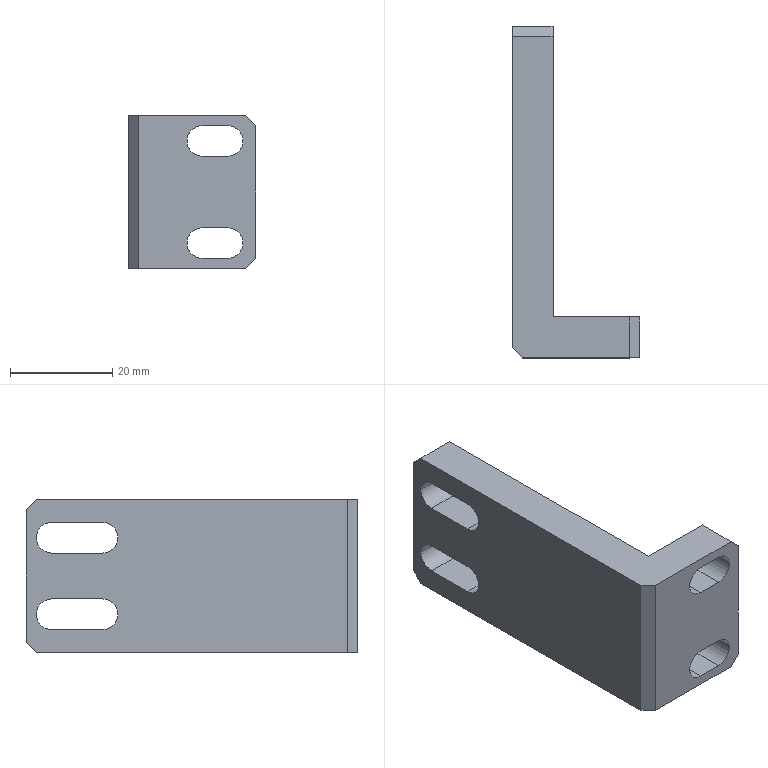Part | STEP file | GLSJ-10-01_default | 1 solid | 31 faces | box 25 x 65 x 30 mm | volume 17211 mm3 | plane 21 | cylinder 10 | commonest cylinder face diameters 6 x10